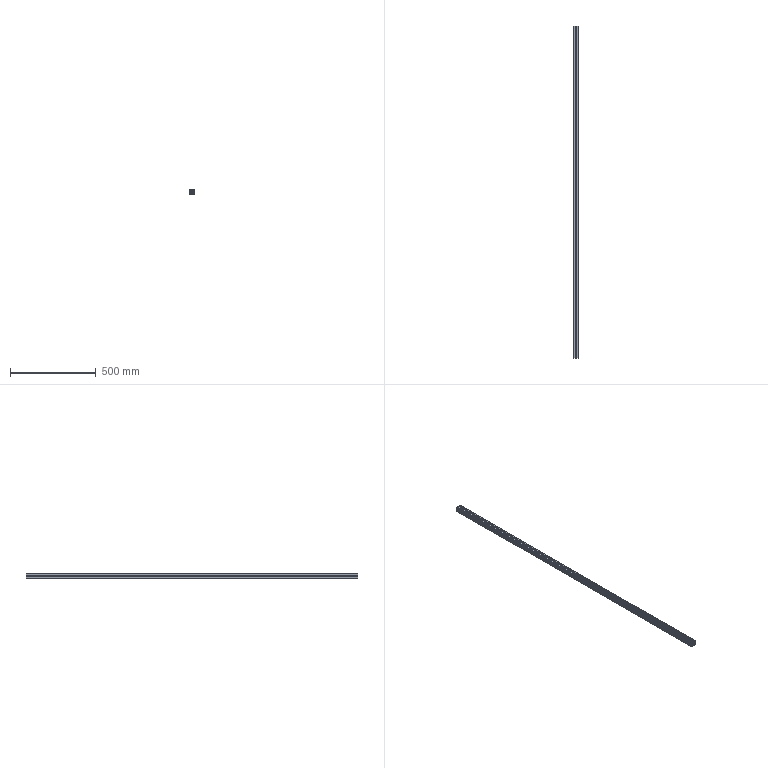Part | SolidWorks | features Extrusion 1, HoleWzd 1 | 1 solid | 108 faces | box 30 x 1940 x 30 mm | volume 644146 mm3 | cylinder 54 | plane 54 | commonest cylinder face diameters 11 x24 6.6 x16 4.2 x8 4 x4 6.8 x2